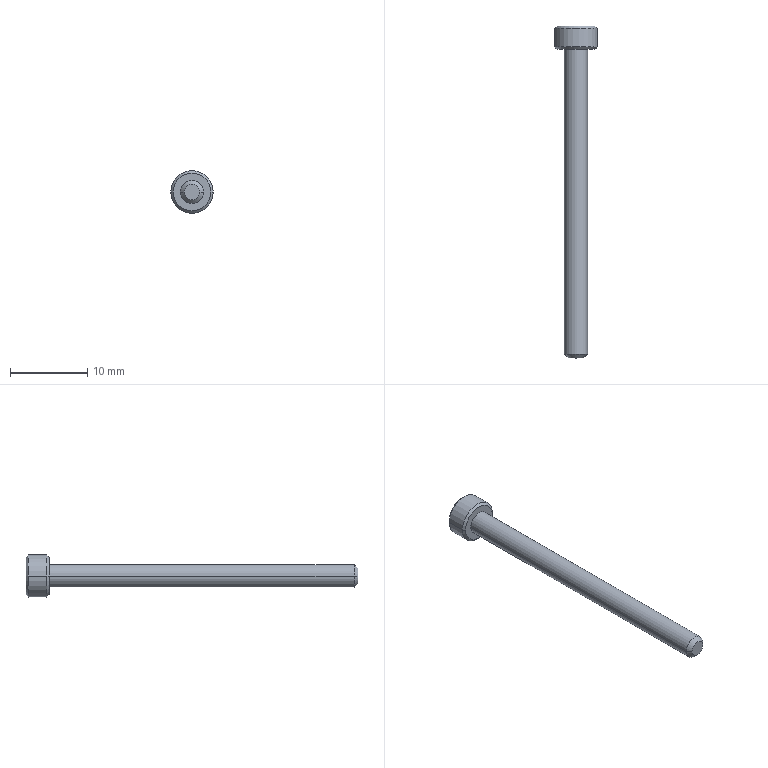Part | STEP file | BB62-M3-40L | 1 solid | 27 faces | box 5.5 x 43 x 5.5 mm | volume 342.731 mm3 | plane 15 | cone 8 | cylinder 4 | commonest cylinder face diameters 3 x2 5.5 x2
STEP:
#1=CARTESIAN_POINT('',(0.,0.8715,0.));
#2=VERTEX_POINT('',#1);
#3=CARTESIAN_POINT('',(1.435,1.7,0.));
#4=VERTEX_POINT('',#3);
#5=CARTESIAN_POINT('',(0.,0.8715,0.));
#6=DIRECTION('',(0.866,0.5,0.));
#7=VECTOR('',#6,1000.);
#8=LINE('',#5,#7);
#9=EDGE_CURVE('',#2,#4,#8,.T.);
#10=ORIENTED_EDGE('',*,*,#9,.F.);
#11=CARTESIAN_POINT('',(-1.435,1.7,0.));
#12=VERTEX_POINT('',#11);
#13=CARTESIAN_POINT('',(0.,0.8715,0.));
#14=DIRECTION('',(-0.866,0.5,0.));
#15=VECTOR('',#14,1000.);
#16=LINE('',#13,#15);
#17=EDGE_CURVE('',#2,#12,#16,.T.);
#18=ORIENTED_EDGE('',*,*,#17,.T.);
#19=CARTESIAN_POINT('',(-1.243,1.7,0.7175));
#20=VERTEX_POINT('',#19);
#21=CARTESIAN_POINT('',(0.,1.7,0.));
#22=DIRECTION('',(0.,-1.,0.));
#23=DIRECTION('',(-1.,0.,0.));
#24=AXIS2_PLACEMENT_3D('',#21,#22,#23);
#25=CIRCLE('',#24,1.435);
#26=EDGE_CURVE('',#20,#12,#25,.T.);
#27=ORIENTED_EDGE('',*,*,#26,.F.);
#28=CARTESIAN_POINT('',(0.,1.7,1.435));
#29=VERTEX_POINT('',#28);
#30=CARTESIAN_POINT('',(0.,1.7,0.));
#31=DIRECTION('',(0.,-1.,0.));
#32=DIRECTION('',(-1.,0.,0.));
#33=AXIS2_PLACEMENT_3D('',#30,#31,#32);
#34=CIRCLE('',#33,1.435);
#35=EDGE_CURVE('',#29,#20,#34,.T.);
#36=ORIENTED_EDGE('',*,*,#35,.F.);
#37=CARTESIAN_POINT('',(1.243,1.7,0.7175));
#38=VERTEX_POINT('',#37);
#39=CARTESIAN_POINT('',(0.,1.7,0.));
#40=DIRECTION('',(0.,-1.,0.));
#41=DIRECTION('',(-1.,0.,0.));
#42=AXIS2_PLACEMENT_3D('',#39,#40,#41);
#43=CIRCLE('',#42,1.435);
#44=EDGE_CURVE('',#38,#29,#43,.T.);
#45=ORIENTED_EDGE('',*,*,#44,.F.);
#46=CARTESIAN_POINT('',(0.,1.7,0.));
#47=DIRECTION('',(0.,-1.,0.));
#48=DIRECTION('',(-1.,0.,0.));
#49=AXIS2_PLACEMENT_3D('',#46,#47,#48);
#50=CIRCLE('',#49,1.435);
#51=EDGE_CURVE('',#4,#38,#50,.T.);
#52=ORIENTED_EDGE('',*,*,#51,.F.);
#53=EDGE_LOOP('',(#10,#18,#27,#36,#45,#52));
#54=FACE_OUTER_BOUND('',#53,.T.);
#55=CARTESIAN_POINT('',(0.,1000.872,0.));
#56=DIRECTION('',(0.,1.,0.));
#57=DIRECTION('',(1.,0.,0.));
#58=AXIS2_PLACEMENT_3D('',#55,#56,#57);
#59=CONICAL_SURFACE('',#58,1732.051,1.047);
#60=ADVANCED_FACE('',(#54),#59,.F.);
#61=CARTESIAN_POINT('',(1.,-40.,0.));
#62=VERTEX_POINT('',#61);
#63=CARTESIAN_POINT('',(-1.,-40.,0.));
#64=VERTEX_POINT('',#63);
#65=CARTESIAN_POINT('',(0.,-40.,0.));
#66=DIRECTION('',(0.,1.,0.));
#67=DIRECTION('',(1.,0.,0.));
#68=AXIS2_PLACEMENT_3D('',#65,#66,#67);
#69=CIRCLE('',#68,1.);
#70=EDGE_CURVE('',#62,#64,#69,.T.);
#71=ORIENTED_EDGE('',*,*,#70,.T.);
#72=CARTESIAN_POINT('',(-1.5,-39.5,0.));
#73=VERTEX_POINT('',#72);
#74=CARTESIAN_POINT('',(-1.,-40.,0.));
#75=DIRECTION('',(-0.7071,0.7071,0.));
#76=VECTOR('',#75,1000.);
#77=LINE('',#74,#76);
#78=EDGE_CURVE('',#64,#73,#77,.T.);
#79=ORIENTED_EDGE('',*,*,#78,.T.);
#80=CARTESIAN_POINT('',(1.5,-39.5,0.));
#81=VERTEX_POINT('',#80);
#82=CARTESIAN_POINT('',(0.,-39.5,0.));
#83=DIRECTION('',(0.,-1.,0.));
#84=DIRECTION('',(-1.,0.,0.));
#85=AXIS2_PLACEMENT_3D('',#82,#83,#84);
#86=CIRCLE('',#85,1.5);
#87=EDGE_CURVE('',#73,#81,#86,.T.);
#88=ORIENTED_EDGE('',*,*,#87,.T.);
#89=CARTESIAN_POINT('',(1.,-40.,0.));
#90=DIRECTION('',(0.7071,0.7071,0.));
#91=VECTOR('',#90,1000.);
#92=LINE('',#89,#91);
#93=EDGE_CURVE('',#62,#81,#92,.T.);
#94=ORIENTED_EDGE('',*,*,#93,.F.);
#95=EDGE_LOOP('',(#71,#79,#88,#94));
#96=FACE_OUTER_BOUND('',#95,.T.);
#97=CARTESIAN_POINT('',(0.,-40.,0.));
#98=DIRECTION('',(0.,1.,0.));
#99=DIRECTION('',(1.,0.,0.));
#100=AXIS2_PLACEMENT_3D('',#97,#98,#99);
#101=CONICAL_SURFACE('',#100,1.,0.7854);
#102=ADVANCED_FACE('',(#96),#101,.T.);
#103=ORIENTED_EDGE('',*,*,#87,.F.);
#104=CARTESIAN_POINT('',(-1.5,0.,0.));
#105=VERTEX_POINT('',#104);
#106=CARTESIAN_POINT('',(-1.5,-39.5,0.));
#107=DIRECTION('',(0.,1.,0.));
#108=VECTOR('',#107,1000.);
#109=LINE('',#106,#108);
#110=EDGE_CURVE('',#73,#105,#109,.T.);
#111=ORIENTED_EDGE('',*,*,#110,.T.);
#112=CARTESIAN_POINT('',(1.5,0.,0.));
#113=VERTEX_POINT('',#112);
#114=CARTESIAN_POINT('',(0.,0.,0.));
#115=DIRECTION('',(0.,-1.,0.));
#116=DIRECTION('',(-1.,0.,0.));
#117=AXIS2_PLACEMENT_3D('',#114,#115,#116);
#118=CIRCLE('',#117,1.5);
#119=EDGE_CURVE('',#105,#113,#118,.T.);
#120=ORIENTED_EDGE('',*,*,#119,.T.);
#121=CARTESIAN_POINT('',(1.5,-39.5,0.));
#122=DIRECTION('',(0.,1.,0.));
#123=VECTOR('',#122,1000.);
#124=LINE('',#121,#123);
#125=EDGE_CURVE('',#81,#113,#124,.T.);
#126=ORIENTED_EDGE('',*,*,#125,.F.);
#127=EDGE_LOOP('',(#103,#111,#120,#126));
#128=FACE_OUTER_BOUND('',#127,.T.);
#129=CARTESIAN_POINT('',(0.,-39.5,0.));
#130=DIRECTION('',(0.,1.,0.));
#131=DIRECTION('',(1.,0.,0.));
#132=AXIS2_PLACEMENT_3D('',#129,#130,#131);
#133=CYLINDRICAL_SURFACE('',#132,1.5);
#134=ADVANCED_FACE('',(#128),#133,.T.);
#135=CARTESIAN_POINT('',(-2.45,3.,0.));
#136=VERTEX_POINT('',#135);
#137=CARTESIAN_POINT('',(2.45,3.,0.));
#138=VERTEX_POINT('',#137);
#139=CARTESIAN_POINT('',(0.,3.,0.));
#140=DIRECTION('',(0.,-1.,0.));
#141=DIRECTION('',(-1.,0.,0.));
#142=AXIS2_PLACEMENT_3D('',#139,#140,#141);
#143=CIRCLE('',#142,2.45);
#144=EDGE_CURVE('',#136,#138,#143,.T.);
#145=ORIENTED_EDGE('',*,*,#144,.T.);
#146=CARTESIAN_POINT('',(2.75,2.7,0.));
#147=VERTEX_POINT('',#146);
#148=CARTESIAN_POINT('',(2.75,2.7,0.));
#149=DIRECTION('',(0.7071,-0.7071,0.));
#150=VECTOR('',#149,1000.);
#151=LINE('',#148,#150);
#152=EDGE_CURVE('',#138,#147,#151,.T.);
#153=ORIENTED_EDGE('',*,*,#152,.T.);
#154=CARTESIAN_POINT('',(-2.75,2.7,0.));
#155=VERTEX_POINT('',#154);
#156=CARTESIAN_POINT('',(0.,2.7,0.));
#157=DIRECTION('',(0.,-1.,0.));
#158=DIRECTION('',(-1.,0.,0.));
#159=AXIS2_PLACEMENT_3D('',#156,#157,#158);
#160=CIRCLE('',#159,2.75);
#161=EDGE_CURVE('',#155,#147,#160,.T.);
#162=ORIENTED_EDGE('',*,*,#161,.F.);
#163=CARTESIAN_POINT('',(-2.75,2.7,0.));
#164=DIRECTION('',(-0.7071,-0.7071,0.));
#165=VECTOR('',#164,1000.);
#166=LINE('',#163,#165);
#167=EDGE_CURVE('',#136,#155,#166,.T.);
#168=ORIENTED_EDGE('',*,*,#167,.F.);
#169=EDGE_LOOP('',(#145,#153,#162,#168));
#170=FACE_OUTER_BOUND('',#169,.T.);
#171=CARTESIAN_POINT('',(0.,2.7,0.));
#172=DIRECTION('',(0.,-1.,0.));
#173=DIRECTION('',(-1.,0.,0.));
#174=AXIS2_PLACEMENT_3D('',#171,#172,#173);
#175=CONICAL_SURFACE('',#174,2.75,0.7854);
#176=ADVANCED_FACE('',(#170),#175,.T.);
#177=ORIENTED_EDGE('',*,*,#161,.T.);
#178=CARTESIAN_POINT('',(2.75,0.3,0.));
#179=VERTEX_POINT('',#178);
#180=CARTESIAN_POINT('',(2.75,1.62,0.));
#181=DIRECTION('',(0.,-1.,0.));
#182=VECTOR('',#181,1000.);
#183=LINE('',#180,#182);
#184=EDGE_CURVE('',#147,#179,#183,.T.);
#185=ORIENTED_EDGE('',*,*,#184,.T.);
#186=CARTESIAN_POINT('',(-2.75,0.3,0.));
#187=VERTEX_POINT('',#186);
#188=CARTESIAN_POINT('',(0.,0.3,0.));
#189=DIRECTION('',(0.,-1.,0.));
#190=DIRECTION('',(-1.,0.,0.));
#191=AXIS2_PLACEMENT_3D('',#188,#189,#190);
#192=CIRCLE('',#191,2.75);
#193=EDGE_CURVE('',#187,#179,#192,.T.);
#194=ORIENTED_EDGE('',*,*,#193,.F.);
#195=CARTESIAN_POINT('',(-2.75,1.62,0.));
#196=DIRECTION('',(0.,-1.,0.));
#197=VECTOR('',#196,1000.);
#198=LINE('',#195,#197);
#199=EDGE_CURVE('',#155,#187,#198,.T.);
#200=ORIENTED_EDGE('',*,*,#199,.F.);
#201=EDGE_LOOP('',(#177,#185,#194,#200));
#202=FACE_OUTER_BOUND('',#201,.T.);
#203=CARTESIAN_POINT('',(0.,1.62,0.));
#204=DIRECTION('',(0.,-1.,0.));
#205=DIRECTION('',(-1.,0.,0.));
#206=AXIS2_PLACEMENT_3D('',#203,#204,#205);
#207=CYLINDRICAL_SURFACE('',#206,2.75);
#208=ADVANCED_FACE('',(#202),#207,.T.);
#209=CARTESIAN_POINT('',(-2.45,0.,0.));
#210=VERTEX_POINT('',#209);
#211=CARTESIAN_POINT('',(2.45,0.,0.));
#212=VERTEX_POINT('',#211);
#213=CARTESIAN_POINT('',(0.,0.,0.));
#214=DIRECTION('',(0.,-1.,0.));
#215=DIRECTION('',(-1.,0.,0.));
#216=AXIS2_PLACEMENT_3D('',#213,#214,#215);
#217=CIRCLE('',#216,2.45);
#218=EDGE_CURVE('',#210,#212,#217,.T.);
#219=ORIENTED_EDGE('',*,*,#218,.F.);
#220=CARTESIAN_POINT('',(-2.45,0.,0.));
#221=DIRECTION('',(-0.7071,0.7071,0.));
#222=VECTOR('',#221,1000.);
#223=LINE('',#220,#222);
#224=EDGE_CURVE('',#210,#187,#223,.T.);
#225=ORIENTED_EDGE('',*,*,#224,.T.);
#226=ORIENTED_EDGE('',*,*,#193,.T.);
#227=CARTESIAN_POINT('',(2.45,0.,0.));
#228=DIRECTION('',(0.7071,0.7071,0.));
#229=VECTOR('',#228,1000.);
#230=LINE('',#227,#229);
#231=EDGE_CURVE('',#212,#179,#230,.T.);
#232=ORIENTED_EDGE('',*,*,#231,.F.);
#233=EDGE_LOOP('',(#219,#225,#226,#232));
#234=FACE_OUTER_BOUND('',#233,.T.);
#235=CARTESIAN_POINT('',(0.,0.,0.));
#236=DIRECTION('',(0.,1.,0.));
#237=DIRECTION('',(1.,0.,0.));
#238=AXIS2_PLACEMENT_3D('',#235,#236,#237);
#239=CONICAL_SURFACE('',#238,2.45,0.7854);
#240=ADVANCED_FACE('',(#234),#239,.T.);
#241=ORIENTED_EDGE('',*,*,#144,.F.);
#242=CARTESIAN_POINT('',(0.,3.,0.));
#243=DIRECTION('',(0.,-1.,0.));
#244=DIRECTION('',(-1.,0.,0.));
#245=AXIS2_PLACEMENT_3D('',#242,#243,#244);
#246=CIRCLE('',#245,2.45);
#247=EDGE_CURVE('',#138,#136,#246,.T.);
#248=ORIENTED_EDGE('',*,*,#247,.F.);
#249=EDGE_LOOP('',(#241,#248));
#250=FACE_OUTER_BOUND('',#249,.T.);
#251=CARTESIAN_POINT('',(0.,3.,-1.435));
#252=VERTEX_POINT('',#251);
#253=CARTESIAN_POINT('',(-1.243,3.,-0.7175));
#254=VERTEX_POINT('',#253);
#255=CARTESIAN_POINT('',(0.,3.,-1.435));
#256=DIRECTION('',(-0.866,0.,0.5));
#257=VECTOR('',#256,1000.);
#258=LINE('',#255,#257);
#259=EDGE_CURVE('',#252,#254,#258,.T.);
#260=ORIENTED_EDGE('',*,*,#259,.F.);
#261=CARTESIAN_POINT('',(1.243,3.,-0.7175));
#262=VERTEX_POINT('',#261);
#263=CARTESIAN_POINT('',(1.243,3.,-0.7175));
#264=DIRECTION('',(-0.866,0.,-0.5));
#265=VECTOR('',#264,1000.);
#266=LINE('',#263,#265);
#267=EDGE_CURVE('',#262,#252,#266,.T.);
#268=ORIENTED_EDGE('',*,*,#267,.F.);
#269=CARTESIAN_POINT('',(1.243,3.,0.7175));
#270=VERTEX_POINT('',#269);
#271=CARTESIAN_POINT('',(1.243,3.,0.7175));
#272=DIRECTION('',(0.,0.,-1.));
#273=VECTOR('',#272,1000.);
#274=LINE('',#271,#273);
#275=EDGE_CURVE('',#270,#262,#274,.T.);
#276=ORIENTED_EDGE('',*,*,#275,.F.);
#277=CARTESIAN_POINT('',(0.,3.,1.435));
#278=VERTEX_POINT('',#277);
#279=CARTESIAN_POINT('',(0.,3.,1.435));
#280=DIRECTION('',(0.866,0.,-0.5));
#281=VECTOR('',#280,1000.);
#282=LINE('',#279,#281);
#283=EDGE_CURVE('',#278,#270,#282,.T.);
#284=ORIENTED_EDGE('',*,*,#283,.F.);
#285=CARTESIAN_POINT('',(-1.243,3.,0.7175));
#286=VERTEX_POINT('',#285);
#287=CARTESIAN_POINT('',(-1.243,3.,0.7175));
#288=DIRECTION('',(0.866,0.,0.5));
#289=VECTOR('',#288,1000.);
#290=LINE('',#287,#289);
#291=EDGE_CURVE('',#286,#278,#290,.T.);
#292=ORIENTED_EDGE('',*,*,#291,.F.);
#293=CARTESIAN_POINT('',(-1.243,3.,-0.7175));
#294=DIRECTION('',(0.,0.,1.));
#295=VECTOR('',#294,1000.);
#296=LINE('',#293,#295);
#297=EDGE_CURVE('',#254,#286,#296,.T.);
#298=ORIENTED_EDGE('',*,*,#297,.F.);
#299=EDGE_LOOP('',(#260,#268,#276,#284,#292,#298));
#300=FACE_BOUND('',#299,.T.);
#301=CARTESIAN_POINT('',(2.45,3.,0.));
#302=DIRECTION('',(0.,1.,0.));
#303=DIRECTION('',(1.,0.,0.));
#304=AXIS2_PLACEMENT_3D('',#301,#302,#303);
#305=PLANE('',#304);
#306=ADVANCED_FACE('',(#250,#300),#305,.T.);
#307=CARTESIAN_POINT('',(0.,0.,0.));
#308=DIRECTION('',(0.,-1.,0.));
#309=DIRECTION('',(-1.,0.,0.));
#310=AXIS2_PLACEMENT_3D('',#307,#308,#309);
#311=CIRCLE('',#310,1.5);
#312=EDGE_CURVE('',#113,#105,#311,.T.);
#313=ORIENTED_EDGE('',*,*,#312,.F.);
#314=ORIENTED_EDGE('',*,*,#119,.F.);
#315=EDGE_LOOP('',(#313,#314));
#316=FACE_BOUND('',#315,.T.);
#317=CARTESIAN_POINT('',(0.,0.,0.));
#318=DIRECTION('',(0.,-1.,0.));
#319=DIRECTION('',(-1.,0.,0.));
#320=AXIS2_PLACEMENT_3D('',#317,#318,#319);
#321=CIRCLE('',#320,2.45);
#322=EDGE_CURVE('',#212,#210,#321,.T.);
#323=ORIENTED_EDGE('',*,*,#322,.T.);
#324=ORIENTED_EDGE('',*,*,#218,.T.);
#325=EDGE_LOOP('',(#323,#324));
#326=FACE_OUTER_BOUND('',#325,.T.);
#327=CARTESIAN_POINT('',(0.,0.,0.));
#328=DIRECTION('',(0.,-1.,0.));
#329=DIRECTION('',(-1.,0.,0.));
#330=AXIS2_PLACEMENT_3D('',#327,#328,#329);
#331=PLANE('',#330);
#332=ADVANCED_FACE('',(#316,#326),#331,.T.);
#333=ORIENTED_EDGE('',*,*,#224,.F.);
#334=ORIENTED_EDGE('',*,*,#322,.F.);
#335=ORIENTED_EDGE('',*,*,#231,.T.);
#336=CARTESIAN_POINT('',(0.,0.3,0.));
#337=DIRECTION('',(0.,-1.,0.));
#338=DIRECTION('',(-1.,0.,0.));
#339=AXIS2_PLACEMENT_3D('',#336,#337,#338);
#340=CIRCLE('',#339,2.75);
#341=EDGE_CURVE('',#179,#187,#340,.T.);
#342=ORIENTED_EDGE('',*,*,#341,.T.);
#343=EDGE_LOOP('',(#333,#334,#335,#342));
#344=FACE_OUTER_BOUND('',#343,.T.);
#345=CARTESIAN_POINT('',(0.,0.,0.));
#346=DIRECTION('',(0.,1.,0.));
#347=DIRECTION('',(1.,0.,0.));
#348=AXIS2_PLACEMENT_3D('',#345,#346,#347);
#349=CONICAL_SURFACE('',#348,2.45,0.7854);
#350=ADVANCED_FACE('',(#344),#349,.T.);
#351=ORIENTED_EDGE('',*,*,#184,.F.);
#352=CARTESIAN_POINT('',(0.,2.7,0.));
#353=DIRECTION('',(0.,-1.,0.));
#354=DIRECTION('',(-1.,0.,0.));
#355=AXIS2_PLACEMENT_3D('',#352,#353,#354);
#356=CIRCLE('',#355,2.75);
#357=EDGE_CURVE('',#147,#155,#356,.T.);
#358=ORIENTED_EDGE('',*,*,#357,.T.);
#359=ORIENTED_EDGE('',*,*,#199,.T.);
#360=ORIENTED_EDGE('',*,*,#341,.F.);
#361=EDGE_LOOP('',(#351,#358,#359,#360));
#362=FACE_OUTER_BOUND('',#361,.T.);
#363=CARTESIAN_POINT('',(0.,1.62,0.));
#364=DIRECTION('',(0.,-1.,0.));
#365=DIRECTION('',(-1.,0.,0.));
#366=AXIS2_PLACEMENT_3D('',#363,#364,#365);
#367=CYLINDRICAL_SURFACE('',#366,2.75);
#368=ADVANCED_FACE('',(#362),#367,.T.);
#369=ORIENTED_EDGE('',*,*,#152,.F.);
#370=ORIENTED_EDGE('',*,*,#247,.T.);
#371=ORIENTED_EDGE('',*,*,#167,.T.);
#372=ORIENTED_EDGE('',*,*,#357,.F.);
#373=EDGE_LOOP('',(#369,#370,#371,#372));
#374=FACE_OUTER_BOUND('',#373,.T.);
#375=CARTESIAN_POINT('',(0.,2.7,0.));
#376=DIRECTION('',(0.,-1.,0.));
#377=DIRECTION('',(-1.,0.,0.));
#378=AXIS2_PLACEMENT_3D('',#375,#376,#377);
#379=CONICAL_SURFACE('',#378,2.75,0.7854);
#380=ADVANCED_FACE('',(#374),#379,.T.);
#381=ORIENTED_EDGE('',*,*,#110,.F.);
#382=CARTESIAN_POINT('',(0.,-39.5,0.));
#383=DIRECTION('',(0.,-1.,0.));
#384=DIRECTION('',(-1.,0.,0.));
#385=AXIS2_PLACEMENT_3D('',#382,#383,#384);
#386=CIRCLE('',#385,1.5);
#387=EDGE_CURVE('',#81,#73,#386,.T.);
#388=ORIENTED_EDGE('',*,*,#387,.F.);
#389=ORIENTED_EDGE('',*,*,#125,.T.);
#390=ORIENTED_EDGE('',*,*,#312,.T.);
#391=EDGE_LOOP('',(#381,#388,#389,#390));
#392=FACE_OUTER_BOUND('',#391,.T.);
#393=CARTESIAN_POINT('',(0.,-39.5,0.));
#394=DIRECTION('',(0.,1.,0.));
#395=DIRECTION('',(1.,0.,0.));
#396=AXIS2_PLACEMENT_3D('',#393,#394,#395);
#397=CYLINDRICAL_SURFACE('',#396,1.5);
#398=ADVANCED_FACE('',(#392),#397,.T.);
#399=ORIENTED_EDGE('',*,*,#70,.F.);
#400=CARTESIAN_POINT('',(0.,-40.,0.));
#401=DIRECTION('',(0.,1.,0.));
#402=DIRECTION('',(1.,0.,0.));
#403=AXIS2_PLACEMENT_3D('',#400,#401,#402);
#404=CIRCLE('',#403,1.);
#405=EDGE_CURVE('',#64,#62,#404,.T.);
#406=ORIENTED_EDGE('',*,*,#405,.F.);
#407=EDGE_LOOP('',(#399,#406));
#408=FACE_OUTER_BOUND('',#407,.T.);
#409=CARTESIAN_POINT('',(0.,-40.,0.));
#410=DIRECTION('',(0.,-1.,0.));
#411=DIRECTION('',(-1.,0.,0.));
#412=AXIS2_PLACEMENT_3D('',#409,#410,#411);
#413=PLANE('',#412);
#414=ADVANCED_FACE('',(#408),#413,.T.);
#415=ORIENTED_EDGE('',*,*,#78,.F.);
#416=ORIENTED_EDGE('',*,*,#405,.T.);
#417=ORIENTED_EDGE('',*,*,#93,.T.);
#418=ORIENTED_EDGE('',*,*,#387,.T.);
#419=EDGE_LOOP('',(#415,#416,#417,#418));
#420=FACE_OUTER_BOUND('',#419,.T.);
#421=CARTESIAN_POINT('',(0.,-40.,0.));
#422=DIRECTION('',(0.,1.,0.));
#423=DIRECTION('',(1.,0.,0.));
#424=AXIS2_PLACEMENT_3D('',#421,#422,#423);
#425=CONICAL_SURFACE('',#424,1.,0.7854);
#426=ADVANCED_FACE('',(#420),#425,.T.);
#427=CARTESIAN_POINT('',(1.243,1.7,-0.7175));
#428=VERTEX_POINT('',#427);
#429=CARTESIAN_POINT('',(0.,1.7,-1.435));
#430=VERTEX_POINT('',#429);
#431=CARTESIAN_POINT('',(1.243,1.7,-0.7175));
#432=DIRECTION('',(-0.866,0.,-0.5));
#433=VECTOR('',#432,1000.);
#434=LINE('',#431,#433);
#435=EDGE_CURVE('',#428,#430,#434,.T.);
#436=ORIENTED_EDGE('',*,*,#435,.F.);
#437=CARTESIAN_POINT('',(1.243,3.,-0.7175));
#438=DIRECTION('',(0.,-1.,0.));
#439=VECTOR('',#438,1000.);
#440=LINE('',#437,#439);
#441=EDGE_CURVE('',#262,#428,#440,.T.);
#442=ORIENTED_EDGE('',*,*,#441,.F.);
#443=ORIENTED_EDGE('',*,*,#267,.T.);
#444=CARTESIAN_POINT('',(0.,3.,-1.435));
#445=DIRECTION('',(0.,-1.,0.));
#446=VECTOR('',#445,1000.);
#447=LINE('',#444,#446);
#448=EDGE_CURVE('',#252,#430,#447,.T.);
#449=ORIENTED_EDGE('',*,*,#448,.T.);
#450=EDGE_LOOP('',(#436,#442,#443,#449));
#451=FACE_OUTER_BOUND('',#450,.T.);
#452=CARTESIAN_POINT('',(1.243,3.,-0.7175));
#453=DIRECTION('',(-0.5,0.,0.866));
#454=DIRECTION('',(0.866,0.,0.5));
#455=AXIS2_PLACEMENT_3D('',#452,#453,#454);
#456=PLANE('',#455);
#457=ADVANCED_FACE('',(#451),#456,.T.);
#458=CARTESIAN_POINT('',(-1.243,1.7,-0.7175));
#459=VERTEX_POINT('',#458);
#460=CARTESIAN_POINT('',(0.,1.7,-1.435));
#461=DIRECTION('',(-0.866,0.,0.5));
#462=VECTOR('',#461,1000.);
#463=LINE('',#460,#462);
#464=EDGE_CURVE('',#430,#459,#463,.T.);
#465=ORIENTED_EDGE('',*,*,#464,.F.);
#466=ORIENTED_EDGE('',*,*,#448,.F.);
#467=ORIENTED_EDGE('',*,*,#259,.T.);
#468=CARTESIAN_POINT('',(-1.243,3.,-0.7175));
#469=DIRECTION('',(0.,-1.,0.));
#470=VECTOR('',#469,1000.);
#471=LINE('',#468,#470);
#472=EDGE_CURVE('',#254,#459,#471,.T.);
#473=ORIENTED_EDGE('',*,*,#472,.T.);
#474=EDGE_LOOP('',(#465,#466,#467,#473));
#475=FACE_OUTER_BOUND('',#474,.T.);
#476=CARTESIAN_POINT('',(0.,3.,-1.435));
#477=DIRECTION('',(0.5,0.,0.866));
#478=DIRECTION('',(0.866,0.,-0.5));
#479=AXIS2_PLACEMENT_3D('',#476,#477,#478);
#480=PLANE('',#479);
#481=ADVANCED_FACE('',(#475),#480,.T.);
#482=CARTESIAN_POINT('',(-1.243,1.7,-0.7175));
#483=DIRECTION('',(0.,0.,1.));
#484=VECTOR('',#483,1000.);
#485=LINE('',#482,#484);
#486=EDGE_CURVE('',#459,#20,#485,.T.);
#487=ORIENTED_EDGE('',*,*,#486,.F.);
#488=ORIENTED_EDGE('',*,*,#472,.F.);
#489=ORIENTED_EDGE('',*,*,#297,.T.);
#490=CARTESIAN_POINT('',(-1.243,3.,0.7175));
#491=DIRECTION('',(0.,-1.,0.));
#492=VECTOR('',#491,1000.);
#493=LINE('',#490,#492);
#494=EDGE_CURVE('',#286,#20,#493,.T.);
#495=ORIENTED_EDGE('',*,*,#494,.T.);
#496=EDGE_LOOP('',(#487,#488,#489,#495));
#497=FACE_OUTER_BOUND('',#496,.T.);
#498=CARTESIAN_POINT('',(-1.243,3.,-0.7175));
#499=DIRECTION('',(1.,0.,0.));
#500=DIRECTION('',(0.,0.,-1.));
#501=AXIS2_PLACEMENT_3D('',#498,#499,#500);
#502=PLANE('',#501);
#503=ADVANCED_FACE('',(#497),#502,.T.);
#504=CARTESIAN_POINT('',(-1.243,1.7,0.7175));
#505=DIRECTION('',(0.866,0.,0.5));
#506=VECTOR('',#505,1000.);
#507=LINE('',#504,#506);
#508=EDGE_CURVE('',#20,#29,#507,.T.);
#509=ORIENTED_EDGE('',*,*,#508,.F.);
#510=ORIENTED_EDGE('',*,*,#494,.F.);
#511=ORIENTED_EDGE('',*,*,#291,.T.);
#512=CARTESIAN_POINT('',(0.,3.,1.435));
#513=DIRECTION('',(0.,-1.,0.));
#514=VECTOR('',#513,1000.);
#515=LINE('',#512,#514);
#516=EDGE_CURVE('',#278,#29,#515,.T.);
#517=ORIENTED_EDGE('',*,*,#516,.T.);
#518=EDGE_LOOP('',(#509,#510,#511,#517));
#519=FACE_OUTER_BOUND('',#518,.T.);
#520=CARTESIAN_POINT('',(-1.243,3.,0.7175));
#521=DIRECTION('',(0.5,0.,-0.866));
#522=DIRECTION('',(-0.866,0.,-0.5));
#523=AXIS2_PLACEMENT_3D('',#520,#521,#522);
#524=PLANE('',#523);
#525=ADVANCED_FACE('',(#519),#524,.T.);
#526=CARTESIAN_POINT('',(0.,1.7,1.435));
#527=DIRECTION('',(0.866,0.,-0.5));
#528=VECTOR('',#527,1000.);
#529=LINE('',#526,#528);
#530=EDGE_CURVE('',#29,#38,#529,.T.);
#531=ORIENTED_EDGE('',*,*,#530,.F.);
#532=ORIENTED_EDGE('',*,*,#516,.F.);
#533=ORIENTED_EDGE('',*,*,#283,.T.);
#534=CARTESIAN_POINT('',(1.243,3.,0.7175));
#535=DIRECTION('',(0.,-1.,0.));
#536=VECTOR('',#535,1000.);
#537=LINE('',#534,#536);
#538=EDGE_CURVE('',#270,#38,#537,.T.);
#539=ORIENTED_EDGE('',*,*,#538,.T.);
#540=EDGE_LOOP('',(#531,#532,#533,#539));
#541=FACE_OUTER_BOUND('',#540,.T.);
#542=CARTESIAN_POINT('',(0.,3.,1.435));
#543=DIRECTION('',(-0.5,0.,-0.866));
#544=DIRECTION('',(-0.866,0.,0.5));
#545=AXIS2_PLACEMENT_3D('',#542,#543,#544);
#546=PLANE('',#545);
#547=ADVANCED_FACE('',(#541),#546,.T.);
#548=CARTESIAN_POINT('',(1.243,1.7,0.7175));
#549=DIRECTION('',(0.,0.,-1.));
#550=VECTOR('',#549,1000.);
#551=LINE('',#548,#550);
#552=EDGE_CURVE('',#38,#428,#551,.T.);
#553=ORIENTED_EDGE('',*,*,#552,.F.);
#554=ORIENTED_EDGE('',*,*,#538,.F.);
#555=ORIENTED_EDGE('',*,*,#275,.T.);
#556=ORIENTED_EDGE('',*,*,#441,.T.);
#557=EDGE_LOOP('',(#553,#554,#555,#556));
#558=FACE_OUTER_BOUND('',#557,.T.);
#559=CARTESIAN_POINT('',(1.243,3.,0.7175));
#560=DIRECTION('',(-1.,0.,0.));
#561=DIRECTION('',(0.,0.,1.));
#562=AXIS2_PLACEMENT_3D('',#559,#560,#561);
#563=PLANE('',#562);
#564=ADVANCED_FACE('',(#558),#563,.T.);
#565=ORIENTED_EDGE('',*,*,#435,.T.);
#566=CARTESIAN_POINT('',(0.,1.7,0.));
#567=DIRECTION('',(0.,-1.,0.));
#568=DIRECTION('',(-1.,0.,0.));
#569=AXIS2_PLACEMENT_3D('',#566,#567,#568);
#570=CIRCLE('',#569,1.435);
#571=EDGE_CURVE('',#430,#428,#570,.T.);
#572=ORIENTED_EDGE('',*,*,#571,.T.);
#573=EDGE_LOOP('',(#565,#572));
#574=FACE_OUTER_BOUND('',#573,.T.);
#575=CARTESIAN_POINT('',(0.,1.7,0.));
#576=DIRECTION('',(0.,1.,0.));
#577=DIRECTION('',(1.,0.,0.));
#578=AXIS2_PLACEMENT_3D('',#575,#576,#577);
#579=PLANE('',#578);
#580=ADVANCED_FACE('',(#574),#579,.F.);
#581=ORIENTED_EDGE('',*,*,#552,.T.);
#582=CARTESIAN_POINT('',(0.,1.7,0.));
#583=DIRECTION('',(0.,-1.,0.));
#584=DIRECTION('',(-1.,0.,0.));
#585=AXIS2_PLACEMENT_3D('',#582,#583,#584);
#586=CIRCLE('',#585,1.435);
#587=EDGE_CURVE('',#428,#4,#586,.T.);
#588=ORIENTED_EDGE('',*,*,#587,.T.);
#589=ORIENTED_EDGE('',*,*,#51,.T.);
#590=EDGE_LOOP('',(#581,#588,#589));
#591=FACE_OUTER_BOUND('',#590,.T.);
#592=CARTESIAN_POINT('',(0.,1.7,0.));
#593=DIRECTION('',(0.,1.,0.));
#594=DIRECTION('',(1.,0.,0.));
#595=AXIS2_PLACEMENT_3D('',#592,#593,#594);
#596=PLANE('',#595);
#597=ADVANCED_FACE('',(#591),#596,.F.);
#598=ORIENTED_EDGE('',*,*,#530,.T.);
#599=ORIENTED_EDGE('',*,*,#44,.T.);
#600=EDGE_LOOP('',(#598,#599));
#601=FACE_OUTER_BOUND('',#600,.T.);
#602=CARTESIAN_POINT('',(0.,1.7,0.));
#603=DIRECTION('',(0.,1.,0.));
#604=DIRECTION('',(1.,0.,0.));
#605=AXIS2_PLACEMENT_3D('',#602,#603,#604);
#606=PLANE('',#605);
#607=ADVANCED_FACE('',(#601),#606,.F.);
#608=ORIENTED_EDGE('',*,*,#508,.T.);
#609=ORIENTED_EDGE('',*,*,#35,.T.);
#610=EDGE_LOOP('',(#608,#609));
#611=FACE_OUTER_BOUND('',#610,.T.);
#612=CARTESIAN_POINT('',(0.,1.7,0.));
#613=DIRECTION('',(0.,1.,0.));
#614=DIRECTION('',(1.,0.,0.));
#615=AXIS2_PLACEMENT_3D('',#612,#613,#614);
#616=PLANE('',#615);
#617=ADVANCED_FACE('',(#611),#616,.F.);
#618=ORIENTED_EDGE('',*,*,#486,.T.);
#619=ORIENTED_EDGE('',*,*,#26,.T.);
#620=CARTESIAN_POINT('',(0.,1.7,0.));
#621=DIRECTION('',(0.,-1.,0.));
#622=DIRECTION('',(-1.,0.,0.));
#623=AXIS2_PLACEMENT_3D('',#620,#621,#622);
#624=CIRCLE('',#623,1.435);
#625=EDGE_CURVE('',#12,#459,#624,.T.);
#626=ORIENTED_EDGE('',*,*,#625,.T.);
#627=EDGE_LOOP('',(#618,#619,#626));
#628=FACE_OUTER_BOUND('',#627,.T.);
#629=CARTESIAN_POINT('',(0.,1.7,0.));
#630=DIRECTION('',(0.,1.,0.));
#631=DIRECTION('',(1.,0.,0.));
#632=AXIS2_PLACEMENT_3D('',#629,#630,#631);
#633=PLANE('',#632);
#634=ADVANCED_FACE('',(#628),#633,.F.);
#635=ORIENTED_EDGE('',*,*,#464,.T.);
#636=CARTESIAN_POINT('',(0.,1.7,0.));
#637=DIRECTION('',(0.,-1.,0.));
#638=DIRECTION('',(-1.,0.,0.));
#639=AXIS2_PLACEMENT_3D('',#636,#637,#638);
#640=CIRCLE('',#639,1.435);
#641=EDGE_CURVE('',#459,#430,#640,.T.);
#642=ORIENTED_EDGE('',*,*,#641,.T.);
#643=EDGE_LOOP('',(#635,#642));
#644=FACE_OUTER_BOUND('',#643,.T.);
#645=CARTESIAN_POINT('',(0.,1.7,0.));
#646=DIRECTION('',(0.,1.,0.));
#647=DIRECTION('',(1.,0.,0.));
#648=AXIS2_PLACEMENT_3D('',#645,#646,#647);
#649=PLANE('',#648);
#650=ADVANCED_FACE('',(#644),#649,.F.);
#651=ORIENTED_EDGE('',*,*,#17,.F.);
#652=ORIENTED_EDGE('',*,*,#9,.T.);
#653=ORIENTED_EDGE('',*,*,#587,.F.);
#654=ORIENTED_EDGE('',*,*,#571,.F.);
#655=ORIENTED_EDGE('',*,*,#641,.F.);
#656=ORIENTED_EDGE('',*,*,#625,.F.);
#657=EDGE_LOOP('',(#651,#652,#653,#654,#655,#656));
#658=FACE_OUTER_BOUND('',#657,.T.);
#659=CARTESIAN_POINT('',(0.,1000.872,0.));
#660=DIRECTION('',(0.,1.,0.));
#661=DIRECTION('',(1.,0.,0.));
#662=AXIS2_PLACEMENT_3D('',#659,#660,#661);
#663=CONICAL_SURFACE('',#662,1732.051,1.047);
#664=ADVANCED_FACE('',(#658),#663,.F.);
#665=CLOSED_SHELL('',(#60,#102,#134,#176,#208,#240,#306,#332,#350,#368,#380,#398,#414,#426,#457,#481,#503,#525,#547,#564,#580,#597,#607,#617,#634,#650,#664));
#666=MANIFOLD_SOLID_BREP('',#665);
#667=CARTESIAN_POINT('',(0.,0.,0.));
#668=DIRECTION('',(0.,0.,1.));
#669=DIRECTION('',(1.,0.,0.));
#670=AXIS2_PLACEMENT_3D('',#667,#668,#669);
#671=(LENGTH_UNIT()NAMED_UNIT(*)SI_UNIT(.MILLI.,.METRE.));
#672=UNCERTAINTY_MEASURE_WITH_UNIT(LENGTH_MEASURE(0.00001),#671,'','');
#673=(NAMED_UNIT(*)PLANE_ANGLE_UNIT()SI_UNIT($,.RADIAN.));
#674=(NAMED_UNIT(*)SI_UNIT($,.STERADIAN.)SOLID_ANGLE_UNIT());
#675=(GEOMETRIC_REPRESENTATION_CONTEXT(3)GLOBAL_UNCERTAINTY_ASSIGNED_CONTEXT((#672))GLOBAL_UNIT_ASSIGNED_CONTEXT((#671,#673,#674))REPRESENTATION_CONTEXT('',''));
#676=ADVANCED_BREP_SHAPE_REPRESENTATION('',(#666,#670),#675);